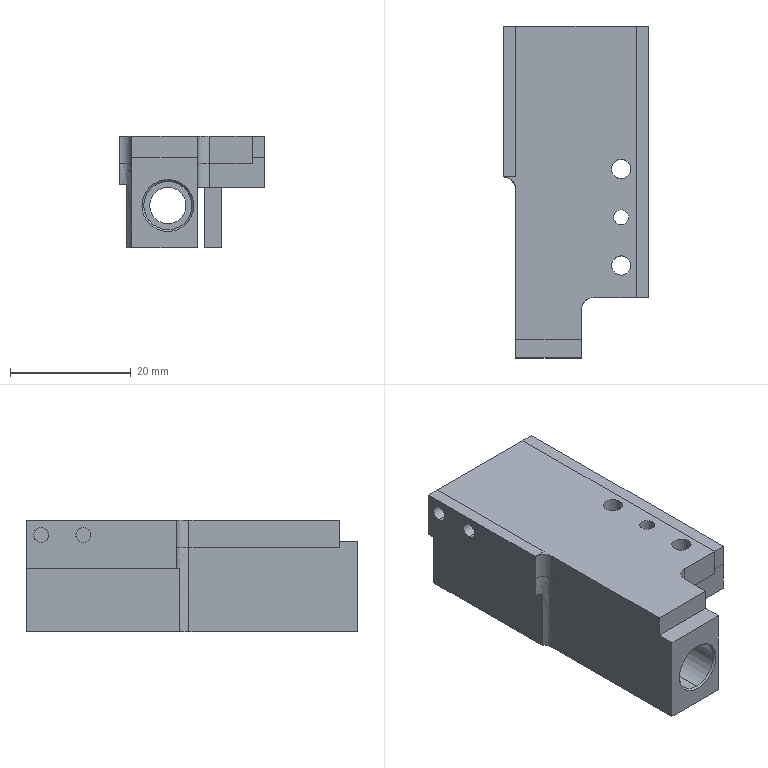NC program | NX | posted with a generic post | part box 24.15 x 55 x 18.5 mm
Whole program:
N10 G17 G21 G94 G90
(DRILLING_COPY_1_COPY , TOOL : D6A45)
N12 T07 M6
N14 G54
N16 G17 G0 G90 X2.5 Y-2.5 B0. C0. S5000 M3
N18 G43 Z30. H7
N20 G94 G81 G98 Z-1.6 F250. R3.
N22 X9.5
N24 G80
N26 G0 X9.5 Y-2.5 Z30.
N28 M5
(DRILLING_COPY_COPY_1_COPY , TOOL : 2.5ZT)
N30 T12 M6
N32 G54
N34 G17 G0 G90 X2.5 Y-2.5 B0. C0. S2000 M3
N36 G43 Z30. H12
N38 G94 G83 G98 Z-4.251 F120. Q2. R3.
N40 X9.5
N42 G80
N44 G0 X9.5 Y-2.5 Z30.
N46 M5
N48 M2